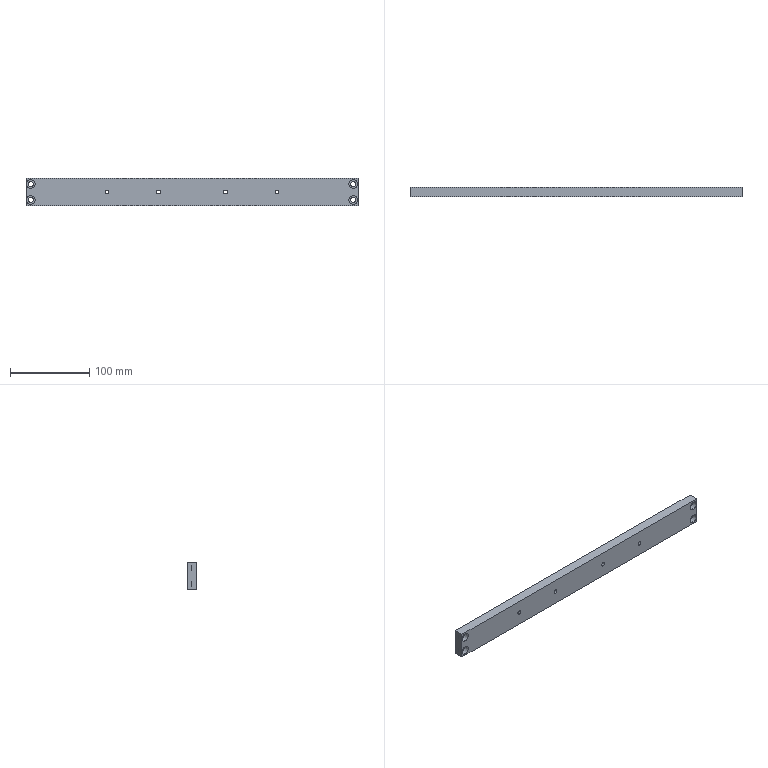Part | SolidWorks | features BaseBody 1 | 1 solid | 34 faces | box 420 x 12 x 35 mm | volume 172258 mm3 | cylinder 24 | plane 10 | commonest cylinder face diameters 5 x8 6.6 x8 11 x8
STEP:
#1=CARTESIAN_POINT('',(107.5,0.,-2.5));
#2=VERTEX_POINT('',#1);
#3=CARTESIAN_POINT('',(107.5,0.,2.5));
#4=VERTEX_POINT('',#3);
#5=CARTESIAN_POINT('',(107.5,0.,0.));
#6=DIRECTION('',(0.,1.,0.));
#7=DIRECTION('',(0.,0.,1.));
#8=AXIS2_PLACEMENT_3D('',#5,#6,#7);
#9=CIRCLE('',#8,2.5);
#10=EDGE_CURVE('',#2,#4,#9,.T.);
#11=ORIENTED_EDGE('',*,*,#10,.F.);
#12=CARTESIAN_POINT('',(107.5,12.,-2.5));
#13=VERTEX_POINT('',#12);
#14=CARTESIAN_POINT('',(107.5,12.,-2.5));
#15=DIRECTION('',(0.,1.,0.));
#16=VECTOR('',#15,1000.);
#17=LINE('',#14,#16);
#18=EDGE_CURVE('',#2,#13,#17,.T.);
#19=ORIENTED_EDGE('',*,*,#18,.T.);
#20=CARTESIAN_POINT('',(107.5,12.,2.5));
#21=VERTEX_POINT('',#20);
#22=CARTESIAN_POINT('',(107.5,12.,0.));
#23=DIRECTION('',(0.,1.,0.));
#24=DIRECTION('',(0.,0.,1.));
#25=AXIS2_PLACEMENT_3D('',#22,#23,#24);
#26=CIRCLE('',#25,2.5);
#27=EDGE_CURVE('',#13,#21,#26,.T.);
#28=ORIENTED_EDGE('',*,*,#27,.T.);
#29=CARTESIAN_POINT('',(107.5,12.,2.5));
#30=DIRECTION('',(0.,1.,0.));
#31=VECTOR('',#30,1000.);
#32=LINE('',#29,#31);
#33=EDGE_CURVE('',#4,#21,#32,.T.);
#34=ORIENTED_EDGE('',*,*,#33,.F.);
#35=EDGE_LOOP('',(#11,#19,#28,#34));
#36=FACE_OUTER_BOUND('',#35,.T.);
#37=CARTESIAN_POINT('',(107.5,12.,0.));
#38=DIRECTION('',(0.,1.,0.));
#39=DIRECTION('',(0.,0.,1.));
#40=AXIS2_PLACEMENT_3D('',#37,#38,#39);
#41=CYLINDRICAL_SURFACE('',#40,2.5);
#42=ADVANCED_FACE('',(#36),#41,.F.);
#43=CARTESIAN_POINT('',(42.5,0.,-2.5));
#44=VERTEX_POINT('',#43);
#45=CARTESIAN_POINT('',(42.5,0.,2.5));
#46=VERTEX_POINT('',#45);
#47=CARTESIAN_POINT('',(42.5,0.,0.));
#48=DIRECTION('',(0.,1.,0.));
#49=DIRECTION('',(0.,0.,1.));
#50=AXIS2_PLACEMENT_3D('',#47,#48,#49);
#51=CIRCLE('',#50,2.5);
#52=EDGE_CURVE('',#44,#46,#51,.T.);
#53=ORIENTED_EDGE('',*,*,#52,.F.);
#54=CARTESIAN_POINT('',(42.5,12.,-2.5));
#55=VERTEX_POINT('',#54);
#56=CARTESIAN_POINT('',(42.5,12.,-2.5));
#57=DIRECTION('',(0.,1.,0.));
#58=VECTOR('',#57,1000.);
#59=LINE('',#56,#58);
#60=EDGE_CURVE('',#44,#55,#59,.T.);
#61=ORIENTED_EDGE('',*,*,#60,.T.);
#62=CARTESIAN_POINT('',(42.5,12.,2.5));
#63=VERTEX_POINT('',#62);
#64=CARTESIAN_POINT('',(42.5,12.,0.));
#65=DIRECTION('',(0.,1.,0.));
#66=DIRECTION('',(0.,0.,1.));
#67=AXIS2_PLACEMENT_3D('',#64,#65,#66);
#68=CIRCLE('',#67,2.5);
#69=EDGE_CURVE('',#55,#63,#68,.T.);
#70=ORIENTED_EDGE('',*,*,#69,.T.);
#71=CARTESIAN_POINT('',(42.5,12.,2.5));
#72=DIRECTION('',(0.,1.,0.));
#73=VECTOR('',#72,1000.);
#74=LINE('',#71,#73);
#75=EDGE_CURVE('',#46,#63,#74,.T.);
#76=ORIENTED_EDGE('',*,*,#75,.F.);
#77=EDGE_LOOP('',(#53,#61,#70,#76));
#78=FACE_OUTER_BOUND('',#77,.T.);
#79=CARTESIAN_POINT('',(42.5,12.,0.));
#80=DIRECTION('',(0.,1.,0.));
#81=DIRECTION('',(0.,0.,1.));
#82=AXIS2_PLACEMENT_3D('',#79,#80,#81);
#83=CYLINDRICAL_SURFACE('',#82,2.5);
#84=ADVANCED_FACE('',(#78),#83,.F.);
#85=CARTESIAN_POINT('',(-42.5,0.,-2.5));
#86=VERTEX_POINT('',#85);
#87=CARTESIAN_POINT('',(-42.5,0.,2.5));
#88=VERTEX_POINT('',#87);
#89=CARTESIAN_POINT('',(-42.5,0.,0.));
#90=DIRECTION('',(0.,1.,0.));
#91=DIRECTION('',(0.,0.,1.));
#92=AXIS2_PLACEMENT_3D('',#89,#90,#91);
#93=CIRCLE('',#92,2.5);
#94=EDGE_CURVE('',#86,#88,#93,.T.);
#95=ORIENTED_EDGE('',*,*,#94,.F.);
#96=CARTESIAN_POINT('',(-42.5,12.,-2.5));
#97=VERTEX_POINT('',#96);
#98=CARTESIAN_POINT('',(-42.5,12.,-2.5));
#99=DIRECTION('',(0.,1.,0.));
#100=VECTOR('',#99,1000.);
#101=LINE('',#98,#100);
#102=EDGE_CURVE('',#86,#97,#101,.T.);
#103=ORIENTED_EDGE('',*,*,#102,.T.);
#104=CARTESIAN_POINT('',(-42.5,12.,2.5));
#105=VERTEX_POINT('',#104);
#106=CARTESIAN_POINT('',(-42.5,12.,0.));
#107=DIRECTION('',(0.,1.,0.));
#108=DIRECTION('',(0.,0.,1.));
#109=AXIS2_PLACEMENT_3D('',#106,#107,#108);
#110=CIRCLE('',#109,2.5);
#111=EDGE_CURVE('',#97,#105,#110,.T.);
#112=ORIENTED_EDGE('',*,*,#111,.T.);
#113=CARTESIAN_POINT('',(-42.5,12.,2.5));
#114=DIRECTION('',(0.,1.,0.));
#115=VECTOR('',#114,1000.);
#116=LINE('',#113,#115);
#117=EDGE_CURVE('',#88,#105,#116,.T.);
#118=ORIENTED_EDGE('',*,*,#117,.F.);
#119=EDGE_LOOP('',(#95,#103,#112,#118));
#120=FACE_OUTER_BOUND('',#119,.T.);
#121=CARTESIAN_POINT('',(-42.5,12.,0.));
#122=DIRECTION('',(0.,1.,0.));
#123=DIRECTION('',(0.,0.,1.));
#124=AXIS2_PLACEMENT_3D('',#121,#122,#123);
#125=CYLINDRICAL_SURFACE('',#124,2.5);
#126=ADVANCED_FACE('',(#120),#125,.F.);
#127=CARTESIAN_POINT('',(-107.5,0.,-2.5));
#128=VERTEX_POINT('',#127);
#129=CARTESIAN_POINT('',(-107.5,0.,2.5));
#130=VERTEX_POINT('',#129);
#131=CARTESIAN_POINT('',(-107.5,0.,0.));
#132=DIRECTION('',(0.,1.,0.));
#133=DIRECTION('',(0.,0.,1.));
#134=AXIS2_PLACEMENT_3D('',#131,#132,#133);
#135=CIRCLE('',#134,2.5);
#136=EDGE_CURVE('',#128,#130,#135,.T.);
#137=ORIENTED_EDGE('',*,*,#136,.F.);
#138=CARTESIAN_POINT('',(-107.5,12.,-2.5));
#139=VERTEX_POINT('',#138);
#140=CARTESIAN_POINT('',(-107.5,12.,-2.5));
#141=DIRECTION('',(0.,1.,0.));
#142=VECTOR('',#141,1000.);
#143=LINE('',#140,#142);
#144=EDGE_CURVE('',#128,#139,#143,.T.);
#145=ORIENTED_EDGE('',*,*,#144,.T.);
#146=CARTESIAN_POINT('',(-107.5,12.,2.5));
#147=VERTEX_POINT('',#146);
#148=CARTESIAN_POINT('',(-107.5,12.,0.));
#149=DIRECTION('',(0.,1.,0.));
#150=DIRECTION('',(0.,0.,1.));
#151=AXIS2_PLACEMENT_3D('',#148,#149,#150);
#152=CIRCLE('',#151,2.5);
#153=EDGE_CURVE('',#139,#147,#152,.T.);
#154=ORIENTED_EDGE('',*,*,#153,.T.);
#155=CARTESIAN_POINT('',(-107.5,12.,2.5));
#156=DIRECTION('',(0.,1.,0.));
#157=VECTOR('',#156,1000.);
#158=LINE('',#155,#157);
#159=EDGE_CURVE('',#130,#147,#158,.T.);
#160=ORIENTED_EDGE('',*,*,#159,.F.);
#161=EDGE_LOOP('',(#137,#145,#154,#160));
#162=FACE_OUTER_BOUND('',#161,.T.);
#163=CARTESIAN_POINT('',(-107.5,12.,0.));
#164=DIRECTION('',(0.,1.,0.));
#165=DIRECTION('',(0.,0.,1.));
#166=AXIS2_PLACEMENT_3D('',#163,#164,#165);
#167=CYLINDRICAL_SURFACE('',#166,2.5);
#168=ADVANCED_FACE('',(#162),#167,.F.);
#169=CARTESIAN_POINT('',(204.,6.4,-4.5));
#170=VERTEX_POINT('',#169);
#171=CARTESIAN_POINT('',(204.,6.4,-15.5));
#172=VERTEX_POINT('',#171);
#173=CARTESIAN_POINT('',(204.,6.4,-10.));
#174=DIRECTION('',(0.,-1.,0.));
#175=DIRECTION('',(0.,0.,-1.));
#176=AXIS2_PLACEMENT_3D('',#173,#174,#175);
#177=CIRCLE('',#176,5.5);
#178=EDGE_CURVE('',#170,#172,#177,.T.);
#179=ORIENTED_EDGE('',*,*,#178,.F.);
#180=CARTESIAN_POINT('',(204.,0.,-4.5));
#181=VERTEX_POINT('',#180);
#182=CARTESIAN_POINT('',(204.,0.,-4.5));
#183=DIRECTION('',(0.,-1.,0.));
#184=VECTOR('',#183,1000.);
#185=LINE('',#182,#184);
#186=EDGE_CURVE('',#170,#181,#185,.T.);
#187=ORIENTED_EDGE('',*,*,#186,.T.);
#188=CARTESIAN_POINT('',(204.,0.,-15.5));
#189=VERTEX_POINT('',#188);
#190=CARTESIAN_POINT('',(204.,0.,-10.));
#191=DIRECTION('',(0.,-1.,0.));
#192=DIRECTION('',(0.,0.,-1.));
#193=AXIS2_PLACEMENT_3D('',#190,#191,#192);
#194=CIRCLE('',#193,5.5);
#195=EDGE_CURVE('',#181,#189,#194,.T.);
#196=ORIENTED_EDGE('',*,*,#195,.T.);
#197=CARTESIAN_POINT('',(204.,0.,-15.5));
#198=DIRECTION('',(0.,-1.,0.));
#199=VECTOR('',#198,1000.);
#200=LINE('',#197,#199);
#201=EDGE_CURVE('',#172,#189,#200,.T.);
#202=ORIENTED_EDGE('',*,*,#201,.F.);
#203=EDGE_LOOP('',(#179,#187,#196,#202));
#204=FACE_OUTER_BOUND('',#203,.T.);
#205=CARTESIAN_POINT('',(204.,0.,-10.));
#206=DIRECTION('',(0.,-1.,0.));
#207=DIRECTION('',(0.,0.,-1.));
#208=AXIS2_PLACEMENT_3D('',#205,#206,#207);
#209=CYLINDRICAL_SURFACE('',#208,5.5);
#210=ADVANCED_FACE('',(#204),#209,.F.);
#211=CARTESIAN_POINT('',(204.,12.,-6.7));
#212=VERTEX_POINT('',#211);
#213=CARTESIAN_POINT('',(204.,12.,-13.3));
#214=VERTEX_POINT('',#213);
#215=CARTESIAN_POINT('',(204.,12.,-10.));
#216=DIRECTION('',(0.,-1.,0.));
#217=DIRECTION('',(0.,0.,-1.));
#218=AXIS2_PLACEMENT_3D('',#215,#216,#217);
#219=CIRCLE('',#218,3.3);
#220=EDGE_CURVE('',#212,#214,#219,.T.);
#221=ORIENTED_EDGE('',*,*,#220,.F.);
#222=CARTESIAN_POINT('',(204.,6.4,-6.7));
#223=VERTEX_POINT('',#222);
#224=CARTESIAN_POINT('',(204.,0.,-6.7));
#225=DIRECTION('',(0.,-1.,0.));
#226=VECTOR('',#225,1000.);
#227=LINE('',#224,#226);
#228=EDGE_CURVE('',#212,#223,#227,.T.);
#229=ORIENTED_EDGE('',*,*,#228,.T.);
#230=CARTESIAN_POINT('',(204.,6.4,-13.3));
#231=VERTEX_POINT('',#230);
#232=CARTESIAN_POINT('',(204.,6.4,-10.));
#233=DIRECTION('',(0.,-1.,0.));
#234=DIRECTION('',(0.,0.,-1.));
#235=AXIS2_PLACEMENT_3D('',#232,#233,#234);
#236=CIRCLE('',#235,3.3);
#237=EDGE_CURVE('',#223,#231,#236,.T.);
#238=ORIENTED_EDGE('',*,*,#237,.T.);
#239=CARTESIAN_POINT('',(204.,0.,-13.3));
#240=DIRECTION('',(0.,-1.,0.));
#241=VECTOR('',#240,1000.);
#242=LINE('',#239,#241);
#243=EDGE_CURVE('',#214,#231,#242,.T.);
#244=ORIENTED_EDGE('',*,*,#243,.F.);
#245=EDGE_LOOP('',(#221,#229,#238,#244));
#246=FACE_OUTER_BOUND('',#245,.T.);
#247=CARTESIAN_POINT('',(204.,0.,-10.));
#248=DIRECTION('',(0.,-1.,0.));
#249=DIRECTION('',(0.,0.,-1.));
#250=AXIS2_PLACEMENT_3D('',#247,#248,#249);
#251=CYLINDRICAL_SURFACE('',#250,3.3);
#252=ADVANCED_FACE('',(#246),#251,.F.);
#253=CARTESIAN_POINT('',(204.,6.4,15.5));
#254=VERTEX_POINT('',#253);
#255=CARTESIAN_POINT('',(204.,6.4,4.5));
#256=VERTEX_POINT('',#255);
#257=CARTESIAN_POINT('',(204.,6.4,10.));
#258=DIRECTION('',(0.,-1.,0.));
#259=DIRECTION('',(0.,0.,-1.));
#260=AXIS2_PLACEMENT_3D('',#257,#258,#259);
#261=CIRCLE('',#260,5.5);
#262=EDGE_CURVE('',#254,#256,#261,.T.);
#263=ORIENTED_EDGE('',*,*,#262,.F.);
#264=CARTESIAN_POINT('',(204.,0.,15.5));
#265=VERTEX_POINT('',#264);
#266=CARTESIAN_POINT('',(204.,0.,15.5));
#267=DIRECTION('',(0.,-1.,0.));
#268=VECTOR('',#267,1000.);
#269=LINE('',#266,#268);
#270=EDGE_CURVE('',#254,#265,#269,.T.);
#271=ORIENTED_EDGE('',*,*,#270,.T.);
#272=CARTESIAN_POINT('',(204.,0.,4.5));
#273=VERTEX_POINT('',#272);
#274=CARTESIAN_POINT('',(204.,0.,10.));
#275=DIRECTION('',(0.,-1.,0.));
#276=DIRECTION('',(0.,0.,-1.));
#277=AXIS2_PLACEMENT_3D('',#274,#275,#276);
#278=CIRCLE('',#277,5.5);
#279=EDGE_CURVE('',#265,#273,#278,.T.);
#280=ORIENTED_EDGE('',*,*,#279,.T.);
#281=CARTESIAN_POINT('',(204.,0.,4.5));
#282=DIRECTION('',(0.,-1.,0.));
#283=VECTOR('',#282,1000.);
#284=LINE('',#281,#283);
#285=EDGE_CURVE('',#256,#273,#284,.T.);
#286=ORIENTED_EDGE('',*,*,#285,.F.);
#287=EDGE_LOOP('',(#263,#271,#280,#286));
#288=FACE_OUTER_BOUND('',#287,.T.);
#289=CARTESIAN_POINT('',(204.,0.,10.));
#290=DIRECTION('',(0.,-1.,0.));
#291=DIRECTION('',(0.,0.,-1.));
#292=AXIS2_PLACEMENT_3D('',#289,#290,#291);
#293=CYLINDRICAL_SURFACE('',#292,5.5);
#294=ADVANCED_FACE('',(#288),#293,.F.);
#295=CARTESIAN_POINT('',(204.,12.,13.3));
#296=VERTEX_POINT('',#295);
#297=CARTESIAN_POINT('',(204.,12.,6.7));
#298=VERTEX_POINT('',#297);
#299=CARTESIAN_POINT('',(204.,12.,10.));
#300=DIRECTION('',(0.,-1.,0.));
#301=DIRECTION('',(0.,0.,-1.));
#302=AXIS2_PLACEMENT_3D('',#299,#300,#301);
#303=CIRCLE('',#302,3.3);
#304=EDGE_CURVE('',#296,#298,#303,.T.);
#305=ORIENTED_EDGE('',*,*,#304,.F.);
#306=CARTESIAN_POINT('',(204.,6.4,13.3));
#307=VERTEX_POINT('',#306);
#308=CARTESIAN_POINT('',(204.,0.,13.3));
#309=DIRECTION('',(0.,-1.,0.));
#310=VECTOR('',#309,1000.);
#311=LINE('',#308,#310);
#312=EDGE_CURVE('',#296,#307,#311,.T.);
#313=ORIENTED_EDGE('',*,*,#312,.T.);
#314=CARTESIAN_POINT('',(204.,6.4,6.7));
#315=VERTEX_POINT('',#314);
#316=CARTESIAN_POINT('',(204.,6.4,10.));
#317=DIRECTION('',(0.,-1.,0.));
#318=DIRECTION('',(0.,0.,-1.));
#319=AXIS2_PLACEMENT_3D('',#316,#317,#318);
#320=CIRCLE('',#319,3.3);
#321=EDGE_CURVE('',#307,#315,#320,.T.);
#322=ORIENTED_EDGE('',*,*,#321,.T.);
#323=CARTESIAN_POINT('',(204.,0.,6.7));
#324=DIRECTION('',(0.,-1.,0.));
#325=VECTOR('',#324,1000.);
#326=LINE('',#323,#325);
#327=EDGE_CURVE('',#298,#315,#326,.T.);
#328=ORIENTED_EDGE('',*,*,#327,.F.);
#329=EDGE_LOOP('',(#305,#313,#322,#328));
#330=FACE_OUTER_BOUND('',#329,.T.);
#331=CARTESIAN_POINT('',(204.,0.,10.));
#332=DIRECTION('',(0.,-1.,0.));
#333=DIRECTION('',(0.,0.,-1.));
#334=AXIS2_PLACEMENT_3D('',#331,#332,#333);
#335=CYLINDRICAL_SURFACE('',#334,3.3);
#336=ADVANCED_FACE('',(#330),#335,.F.);
#337=CARTESIAN_POINT('',(-204.,6.4,-4.5));
#338=VERTEX_POINT('',#337);
#339=CARTESIAN_POINT('',(-204.,6.4,-15.5));
#340=VERTEX_POINT('',#339);
#341=CARTESIAN_POINT('',(-204.,6.4,-10.));
#342=DIRECTION('',(0.,-1.,0.));
#343=DIRECTION('',(0.,0.,-1.));
#344=AXIS2_PLACEMENT_3D('',#341,#342,#343);
#345=CIRCLE('',#344,5.5);
#346=EDGE_CURVE('',#338,#340,#345,.T.);
#347=ORIENTED_EDGE('',*,*,#346,.F.);
#348=CARTESIAN_POINT('',(-204.,0.,-4.5));
#349=VERTEX_POINT('',#348);
#350=CARTESIAN_POINT('',(-204.,0.,-4.5));
#351=DIRECTION('',(0.,-1.,0.));
#352=VECTOR('',#351,1000.);
#353=LINE('',#350,#352);
#354=EDGE_CURVE('',#338,#349,#353,.T.);
#355=ORIENTED_EDGE('',*,*,#354,.T.);
#356=CARTESIAN_POINT('',(-204.,0.,-15.5));
#357=VERTEX_POINT('',#356);
#358=CARTESIAN_POINT('',(-204.,0.,-10.));
#359=DIRECTION('',(0.,-1.,0.));
#360=DIRECTION('',(0.,0.,-1.));
#361=AXIS2_PLACEMENT_3D('',#358,#359,#360);
#362=CIRCLE('',#361,5.5);
#363=EDGE_CURVE('',#349,#357,#362,.T.);
#364=ORIENTED_EDGE('',*,*,#363,.T.);
#365=CARTESIAN_POINT('',(-204.,0.,-15.5));
#366=DIRECTION('',(0.,-1.,0.));
#367=VECTOR('',#366,1000.);
#368=LINE('',#365,#367);
#369=EDGE_CURVE('',#340,#357,#368,.T.);
#370=ORIENTED_EDGE('',*,*,#369,.F.);
#371=EDGE_LOOP('',(#347,#355,#364,#370));
#372=FACE_OUTER_BOUND('',#371,.T.);
#373=CARTESIAN_POINT('',(-204.,0.,-10.));
#374=DIRECTION('',(0.,-1.,0.));
#375=DIRECTION('',(0.,0.,-1.));
#376=AXIS2_PLACEMENT_3D('',#373,#374,#375);
#377=CYLINDRICAL_SURFACE('',#376,5.5);
#378=ADVANCED_FACE('',(#372),#377,.F.);
#379=CARTESIAN_POINT('',(-204.,12.,-6.7));
#380=VERTEX_POINT('',#379);
#381=CARTESIAN_POINT('',(-204.,12.,-13.3));
#382=VERTEX_POINT('',#381);
#383=CARTESIAN_POINT('',(-204.,12.,-10.));
#384=DIRECTION('',(0.,-1.,0.));
#385=DIRECTION('',(0.,0.,-1.));
#386=AXIS2_PLACEMENT_3D('',#383,#384,#385);
#387=CIRCLE('',#386,3.3);
#388=EDGE_CURVE('',#380,#382,#387,.T.);
#389=ORIENTED_EDGE('',*,*,#388,.F.);
#390=CARTESIAN_POINT('',(-204.,6.4,-6.7));
#391=VERTEX_POINT('',#390);
#392=CARTESIAN_POINT('',(-204.,0.,-6.7));
#393=DIRECTION('',(0.,-1.,0.));
#394=VECTOR('',#393,1000.);
#395=LINE('',#392,#394);
#396=EDGE_CURVE('',#380,#391,#395,.T.);
#397=ORIENTED_EDGE('',*,*,#396,.T.);
#398=CARTESIAN_POINT('',(-204.,6.4,-13.3));
#399=VERTEX_POINT('',#398);
#400=CARTESIAN_POINT('',(-204.,6.4,-10.));
#401=DIRECTION('',(0.,-1.,0.));
#402=DIRECTION('',(0.,0.,-1.));
#403=AXIS2_PLACEMENT_3D('',#400,#401,#402);
#404=CIRCLE('',#403,3.3);
#405=EDGE_CURVE('',#391,#399,#404,.T.);
#406=ORIENTED_EDGE('',*,*,#405,.T.);
#407=CARTESIAN_POINT('',(-204.,0.,-13.3));
#408=DIRECTION('',(0.,-1.,0.));
#409=VECTOR('',#408,1000.);
#410=LINE('',#407,#409);
#411=EDGE_CURVE('',#382,#399,#410,.T.);
#412=ORIENTED_EDGE('',*,*,#411,.F.);
#413=EDGE_LOOP('',(#389,#397,#406,#412));
#414=FACE_OUTER_BOUND('',#413,.T.);
#415=CARTESIAN_POINT('',(-204.,0.,-10.));
#416=DIRECTION('',(0.,-1.,0.));
#417=DIRECTION('',(0.,0.,-1.));
#418=AXIS2_PLACEMENT_3D('',#415,#416,#417);
#419=CYLINDRICAL_SURFACE('',#418,3.3);
#420=ADVANCED_FACE('',(#414),#419,.F.);
#421=CARTESIAN_POINT('',(-204.,6.4,15.5));
#422=VERTEX_POINT('',#421);
#423=CARTESIAN_POINT('',(-204.,6.4,4.5));
#424=VERTEX_POINT('',#423);
#425=CARTESIAN_POINT('',(-204.,6.4,10.));
#426=DIRECTION('',(0.,-1.,0.));
#427=DIRECTION('',(0.,0.,-1.));
#428=AXIS2_PLACEMENT_3D('',#425,#426,#427);
#429=CIRCLE('',#428,5.5);
#430=EDGE_CURVE('',#422,#424,#429,.T.);
#431=ORIENTED_EDGE('',*,*,#430,.F.);
#432=CARTESIAN_POINT('',(-204.,0.,15.5));
#433=VERTEX_POINT('',#432);
#434=CARTESIAN_POINT('',(-204.,0.,15.5));
#435=DIRECTION('',(0.,-1.,0.));
#436=VECTOR('',#435,1000.);
#437=LINE('',#434,#436);
#438=EDGE_CURVE('',#422,#433,#437,.T.);
#439=ORIENTED_EDGE('',*,*,#438,.T.);
#440=CARTESIAN_POINT('',(-204.,0.,4.5));
#441=VERTEX_POINT('',#440);
#442=CARTESIAN_POINT('',(-204.,0.,10.));
#443=DIRECTION('',(0.,-1.,0.));
#444=DIRECTION('',(0.,0.,-1.));
#445=AXIS2_PLACEMENT_3D('',#442,#443,#444);
#446=CIRCLE('',#445,5.5);
#447=EDGE_CURVE('',#433,#441,#446,.T.);
#448=ORIENTED_EDGE('',*,*,#447,.T.);
#449=CARTESIAN_POINT('',(-204.,0.,4.5));
#450=DIRECTION('',(0.,-1.,0.));
#451=VECTOR('',#450,1000.);
#452=LINE('',#449,#451);
#453=EDGE_CURVE('',#424,#441,#452,.T.);
#454=ORIENTED_EDGE('',*,*,#453,.F.);
#455=EDGE_LOOP('',(#431,#439,#448,#454));
#456=FACE_OUTER_BOUND('',#455,.T.);
#457=CARTESIAN_POINT('',(-204.,0.,10.));
#458=DIRECTION('',(0.,-1.,0.));
#459=DIRECTION('',(0.,0.,-1.));
#460=AXIS2_PLACEMENT_3D('',#457,#458,#459);
#461=CYLINDRICAL_SURFACE('',#460,5.5);
#462=ADVANCED_FACE('',(#456),#461,.F.);
#463=CARTESIAN_POINT('',(-204.,12.,13.3));
#464=VERTEX_POINT('',#463);
#465=CARTESIAN_POINT('',(-204.,12.,6.7));
#466=VERTEX_POINT('',#465);
#467=CARTESIAN_POINT('',(-204.,12.,10.));
#468=DIRECTION('',(0.,-1.,0.));
#469=DIRECTION('',(0.,0.,-1.));
#470=AXIS2_PLACEMENT_3D('',#467,#468,#469);
#471=CIRCLE('',#470,3.3);
#472=EDGE_CURVE('',#464,#466,#471,.T.);
#473=ORIENTED_EDGE('',*,*,#472,.F.);
#474=CARTESIAN_POINT('',(-204.,6.4,13.3));
#475=VERTEX_POINT('',#474);
#476=CARTESIAN_POINT('',(-204.,0.,13.3));
#477=DIRECTION('',(0.,-1.,0.));
#478=VECTOR('',#477,1000.);
#479=LINE('',#476,#478);
#480=EDGE_CURVE('',#464,#475,#479,.T.);
#481=ORIENTED_EDGE('',*,*,#480,.T.);
#482=CARTESIAN_POINT('',(-204.,6.4,6.7));
#483=VERTEX_POINT('',#482);
#484=CARTESIAN_POINT('',(-204.,6.4,10.));
#485=DIRECTION('',(0.,-1.,0.));
#486=DIRECTION('',(0.,0.,-1.));
#487=AXIS2_PLACEMENT_3D('',#484,#485,#486);
#488=CIRCLE('',#487,3.3);
#489=EDGE_CURVE('',#475,#483,#488,.T.);
#490=ORIENTED_EDGE('',*,*,#489,.T.);
#491=CARTESIAN_POINT('',(-204.,0.,6.7));
#492=DIRECTION('',(0.,-1.,0.));
#493=VECTOR('',#492,1000.);
#494=LINE('',#491,#493);
#495=EDGE_CURVE('',#466,#483,#494,.T.);
#496=ORIENTED_EDGE('',*,*,#495,.F.);
#497=EDGE_LOOP('',(#473,#481,#490,#496));
#498=FACE_OUTER_BOUND('',#497,.T.);
#499=CARTESIAN_POINT('',(-204.,0.,10.));
#500=DIRECTION('',(0.,-1.,0.));
#501=DIRECTION('',(0.,0.,-1.));
#502=AXIS2_PLACEMENT_3D('',#499,#500,#501);
#503=CYLINDRICAL_SURFACE('',#502,3.3);
#504=ADVANCED_FACE('',(#498),#503,.F.);
#505=CARTESIAN_POINT('',(-210.,0.,-17.5));
#506=VERTEX_POINT('',#505);
#507=CARTESIAN_POINT('',(-210.,0.,17.5));
#508=VERTEX_POINT('',#507);
#509=CARTESIAN_POINT('',(-210.,0.,-17.5));
#510=DIRECTION('',(0.,0.,1.));
#511=VECTOR('',#510,1000.);
#512=LINE('',#509,#511);
#513=EDGE_CURVE('',#506,#508,#512,.T.);
#514=ORIENTED_EDGE('',*,*,#513,.T.);
#515=CARTESIAN_POINT('',(-210.,12.,17.5));
#516=VERTEX_POINT('',#515);
#517=CARTESIAN_POINT('',(-210.,12.,17.5));
#518=DIRECTION('',(0.,-1.,0.));
#519=VECTOR('',#518,1000.);
#520=LINE('',#517,#519);
#521=EDGE_CURVE('',#516,#508,#520,.T.);
#522=ORIENTED_EDGE('',*,*,#521,.F.);
#523=CARTESIAN_POINT('',(-210.,12.,-17.5));
#524=VERTEX_POINT('',#523);
#525=CARTESIAN_POINT('',(-210.,12.,-17.5));
#526=DIRECTION('',(0.,0.,1.));
#527=VECTOR('',#526,1000.);
#528=LINE('',#525,#527);
#529=EDGE_CURVE('',#524,#516,#528,.T.);
#530=ORIENTED_EDGE('',*,*,#529,.F.);
#531=CARTESIAN_POINT('',(-210.,12.,-17.5));
#532=DIRECTION('',(0.,-1.,0.));
#533=VECTOR('',#532,1000.);
#534=LINE('',#531,#533);
#535=EDGE_CURVE('',#524,#506,#534,.T.);
#536=ORIENTED_EDGE('',*,*,#535,.T.);
#537=EDGE_LOOP('',(#514,#522,#530,#536));
#538=FACE_OUTER_BOUND('',#537,.T.);
#539=CARTESIAN_POINT('',(-210.,12.,-17.5));
#540=DIRECTION('',(1.,0.,0.));
#541=DIRECTION('',(0.,0.,-1.));
#542=AXIS2_PLACEMENT_3D('',#539,#540,#541);
#543=PLANE('',#542);
#544=ADVANCED_FACE('',(#538),#543,.F.);
#545=CARTESIAN_POINT('',(210.,0.,17.5));
#546=VERTEX_POINT('',#545);
#547=CARTESIAN_POINT('',(210.,0.,17.5));
#548=DIRECTION('',(1.,0.,0.));
#549=VECTOR('',#548,1000.);
#550=LINE('',#547,#549);
#551=EDGE_CURVE('',#508,#546,#550,.T.);
#552=ORIENTED_EDGE('',*,*,#551,.T.);
#553=CARTESIAN_POINT('',(210.,12.,17.5));
#554=VERTEX_POINT('',#553);
#555=CARTESIAN_POINT('',(210.,12.,17.5));
#556=DIRECTION('',(0.,-1.,0.));
#557=VECTOR('',#556,1000.);
#558=LINE('',#555,#557);
#559=EDGE_CURVE('',#554,#546,#558,.T.);
#560=ORIENTED_EDGE('',*,*,#559,.F.);
#561=CARTESIAN_POINT('',(210.,12.,17.5));
#562=DIRECTION('',(1.,0.,0.));
#563=VECTOR('',#562,1000.);
#564=LINE('',#561,#563);
#565=EDGE_CURVE('',#516,#554,#564,.T.);
#566=ORIENTED_EDGE('',*,*,#565,.F.);
#567=ORIENTED_EDGE('',*,*,#521,.T.);
#568=EDGE_LOOP('',(#552,#560,#566,#567));
#569=FACE_OUTER_BOUND('',#568,.T.);
#570=CARTESIAN_POINT('',(210.,12.,17.5));
#571=DIRECTION('',(0.,0.,-1.));
#572=DIRECTION('',(-1.,0.,0.));
#573=AXIS2_PLACEMENT_3D('',#570,#571,#572);
#574=PLANE('',#573);
#575=ADVANCED_FACE('',(#569),#574,.F.);
#576=CARTESIAN_POINT('',(210.,0.,-17.5));
#577=VERTEX_POINT('',#576);
#578=CARTESIAN_POINT('',(210.,0.,-17.5));
#579=DIRECTION('',(0.,0.,-1.));
#580=VECTOR('',#579,1000.);
#581=LINE('',#578,#580);
#582=EDGE_CURVE('',#546,#577,#581,.T.);
#583=ORIENTED_EDGE('',*,*,#582,.T.);
#584=CARTESIAN_POINT('',(210.,12.,-17.5));
#585=VERTEX_POINT('',#584);
#586=CARTESIAN_POINT('',(210.,12.,-17.5));
#587=DIRECTION('',(0.,-1.,0.));
#588=VECTOR('',#587,1000.);
#589=LINE('',#586,#588);
#590=EDGE_CURVE('',#585,#577,#589,.T.);
#591=ORIENTED_EDGE('',*,*,#590,.F.);
#592=CARTESIAN_POINT('',(210.,12.,-17.5));
#593=DIRECTION('',(0.,0.,-1.));
#594=VECTOR('',#593,1000.);
#595=LINE('',#592,#594);
#596=EDGE_CURVE('',#554,#585,#595,.T.);
#597=ORIENTED_EDGE('',*,*,#596,.F.);
#598=ORIENTED_EDGE('',*,*,#559,.T.);
#599=EDGE_LOOP('',(#583,#591,#597,#598));
#600=FACE_OUTER_BOUND('',#599,.T.);
#601=CARTESIAN_POINT('',(210.,12.,-17.5));
#602=DIRECTION('',(-1.,0.,0.));
#603=DIRECTION('',(0.,0.,1.));
#604=AXIS2_PLACEMENT_3D('',#601,#602,#603);
#605=PLANE('',#604);
#606=ADVANCED_FACE('',(#600),#605,.F.);
#607=CARTESIAN_POINT('',(210.,0.,-17.5));
#608=DIRECTION('',(-1.,0.,0.));
#609=VECTOR('',#608,1000.);
#610=LINE('',#607,#609);
#611=EDGE_CURVE('',#577,#506,#610,.T.);
#612=ORIENTED_EDGE('',*,*,#611,.T.);
#613=ORIENTED_EDGE('',*,*,#535,.F.);
#614=CARTESIAN_POINT('',(210.,12.,-17.5));
#615=DIRECTION('',(-1.,0.,0.));
#616=VECTOR('',#615,1000.);
#617=LINE('',#614,#616);
#618=EDGE_CURVE('',#585,#524,#617,.T.);
#619=ORIENTED_EDGE('',*,*,#618,.F.);
#620=ORIENTED_EDGE('',*,*,#590,.T.);
#621=EDGE_LOOP('',(#612,#613,#619,#620));
#622=FACE_OUTER_BOUND('',#621,.T.);
#623=CARTESIAN_POINT('',(210.,12.,-17.5));
#624=DIRECTION('',(0.,0.,1.));
#625=DIRECTION('',(1.,0.,0.));
#626=AXIS2_PLACEMENT_3D('',#623,#624,#625);
#627=PLANE('',#626);
#628=ADVANCED_FACE('',(#622),#627,.F.);
#629=CARTESIAN_POINT('',(107.5,12.,0.));
#630=DIRECTION('',(0.,1.,0.));
#631=DIRECTION('',(0.,0.,1.));
#632=AXIS2_PLACEMENT_3D('',#629,#630,#631);
#633=CIRCLE('',#632,2.5);
#634=EDGE_CURVE('',#21,#13,#633,.T.);
#635=ORIENTED_EDGE('',*,*,#634,.F.);
#636=ORIENTED_EDGE('',*,*,#27,.F.);
#637=EDGE_LOOP('',(#635,#636));
#638=FACE_BOUND('',#637,.T.);
#639=CARTESIAN_POINT('',(42.5,12.,0.));
#640=DIRECTION('',(0.,1.,0.));
#641=DIRECTION('',(0.,0.,1.));
#642=AXIS2_PLACEMENT_3D('',#639,#640,#641);
#643=CIRCLE('',#642,2.5);
#644=EDGE_CURVE('',#63,#55,#643,.T.);
#645=ORIENTED_EDGE('',*,*,#644,.F.);
#646=ORIENTED_EDGE('',*,*,#69,.F.);
#647=EDGE_LOOP('',(#645,#646));
#648=FACE_BOUND('',#647,.T.);
#649=CARTESIAN_POINT('',(-42.5,12.,0.));
#650=DIRECTION('',(0.,1.,0.));
#651=DIRECTION('',(0.,0.,1.));
#652=AXIS2_PLACEMENT_3D('',#649,#650,#651);
#653=CIRCLE('',#652,2.5);
#654=EDGE_CURVE('',#105,#97,#653,.T.);
#655=ORIENTED_EDGE('',*,*,#654,.F.);
#656=ORIENTED_EDGE('',*,*,#111,.F.);
#657=EDGE_LOOP('',(#655,#656));
#658=FACE_BOUND('',#657,.T.);
#659=CARTESIAN_POINT('',(-107.5,12.,0.));
#660=DIRECTION('',(0.,1.,0.));
#661=DIRECTION('',(0.,0.,1.));
#662=AXIS2_PLACEMENT_3D('',#659,#660,#661);
#663=CIRCLE('',#662,2.5);
#664=EDGE_CURVE('',#147,#139,#663,.T.);
#665=ORIENTED_EDGE('',*,*,#664,.F.);
#666=ORIENTED_EDGE('',*,*,#153,.F.);
#667=EDGE_LOOP('',(#665,#666));
#668=FACE_BOUND('',#667,.T.);
#669=CARTESIAN_POINT('',(204.,12.,-10.));
#670=DIRECTION('',(0.,-1.,0.));
#671=DIRECTION('',(0.,0.,-1.));
#672=AXIS2_PLACEMENT_3D('',#669,#670,#671);
#673=CIRCLE('',#672,3.3);
#674=EDGE_CURVE('',#214,#212,#673,.T.);
#675=ORIENTED_EDGE('',*,*,#674,.T.);
#676=ORIENTED_EDGE('',*,*,#220,.T.);
#677=EDGE_LOOP('',(#675,#676));
#678=FACE_BOUND('',#677,.T.);
#679=CARTESIAN_POINT('',(204.,12.,10.));
#680=DIRECTION('',(0.,-1.,0.));
#681=DIRECTION('',(0.,0.,-1.));
#682=AXIS2_PLACEMENT_3D('',#679,#680,#681);
#683=CIRCLE('',#682,3.3);
#684=EDGE_CURVE('',#298,#296,#683,.T.);
#685=ORIENTED_EDGE('',*,*,#684,.T.);
#686=ORIENTED_EDGE('',*,*,#304,.T.);
#687=EDGE_LOOP('',(#685,#686));
#688=FACE_BOUND('',#687,.T.);
#689=CARTESIAN_POINT('',(-204.,12.,-10.));
#690=DIRECTION('',(0.,-1.,0.));
#691=DIRECTION('',(0.,0.,-1.));
#692=AXIS2_PLACEMENT_3D('',#689,#690,#691);
#693=CIRCLE('',#692,3.3);
#694=EDGE_CURVE('',#382,#380,#693,.T.);
#695=ORIENTED_EDGE('',*,*,#694,.T.);
#696=ORIENTED_EDGE('',*,*,#388,.T.);
#697=EDGE_LOOP('',(#695,#696));
#698=FACE_BOUND('',#697,.T.);
#699=CARTESIAN_POINT('',(-204.,12.,10.));
#700=DIRECTION('',(0.,-1.,0.));
#701=DIRECTION('',(0.,0.,-1.));
#702=AXIS2_PLACEMENT_3D('',#699,#700,#701);
#703=CIRCLE('',#702,3.3);
#704=EDGE_CURVE('',#466,#464,#703,.T.);
#705=ORIENTED_EDGE('',*,*,#704,.T.);
#706=ORIENTED_EDGE('',*,*,#472,.T.);
#707=EDGE_LOOP('',(#705,#706));
#708=FACE_BOUND('',#707,.T.);
#709=ORIENTED_EDGE('',*,*,#529,.T.);
#710=ORIENTED_EDGE('',*,*,#565,.T.);
#711=ORIENTED_EDGE('',*,*,#596,.T.);
#712=ORIENTED_EDGE('',*,*,#618,.T.);
#713=EDGE_LOOP('',(#709,#710,#711,#712));
#714=FACE_OUTER_BOUND('',#713,.T.);
#715=CARTESIAN_POINT('',(0.,12.,0.));
#716=DIRECTION('',(0.,-1.,0.));
#717=DIRECTION('',(0.,0.,-1.));
#718=AXIS2_PLACEMENT_3D('',#715,#716,#717);
#719=PLANE('',#718);
#720=ADVANCED_FACE('',(#638,#648,#658,#668,#678,#688,#698,#708,#714),#719,.F.);
#721=CARTESIAN_POINT('',(107.5,0.,0.));
#722=DIRECTION('',(0.,1.,0.));
#723=DIRECTION('',(0.,0.,1.));
#724=AXIS2_PLACEMENT_3D('',#721,#722,#723);
#725=CIRCLE('',#724,2.5);
#726=EDGE_CURVE('',#4,#2,#725,.T.);
#727=ORIENTED_EDGE('',*,*,#726,.T.);
#728=ORIENTED_EDGE('',*,*,#10,.T.);
#729=EDGE_LOOP('',(#727,#728));
#730=FACE_BOUND('',#729,.T.);
#731=CARTESIAN_POINT('',(42.5,0.,0.));
#732=DIRECTION('',(0.,1.,0.));
#733=DIRECTION('',(0.,0.,1.));
#734=AXIS2_PLACEMENT_3D('',#731,#732,#733);
#735=CIRCLE('',#734,2.5);
#736=EDGE_CURVE('',#46,#44,#735,.T.);
#737=ORIENTED_EDGE('',*,*,#736,.T.);
#738=ORIENTED_EDGE('',*,*,#52,.T.);
#739=EDGE_LOOP('',(#737,#738));
#740=FACE_BOUND('',#739,.T.);
#741=CARTESIAN_POINT('',(-42.5,0.,0.));
#742=DIRECTION('',(0.,1.,0.));
#743=DIRECTION('',(0.,0.,1.));
#744=AXIS2_PLACEMENT_3D('',#741,#742,#743);
#745=CIRCLE('',#744,2.5);
#746=EDGE_CURVE('',#88,#86,#745,.T.);
#747=ORIENTED_EDGE('',*,*,#746,.T.);
#748=ORIENTED_EDGE('',*,*,#94,.T.);
#749=EDGE_LOOP('',(#747,#748));
#750=FACE_BOUND('',#749,.T.);
#751=CARTESIAN_POINT('',(-107.5,0.,0.));
#752=DIRECTION('',(0.,1.,0.));
#753=DIRECTION('',(0.,0.,1.));
#754=AXIS2_PLACEMENT_3D('',#751,#752,#753);
#755=CIRCLE('',#754,2.5);
#756=EDGE_CURVE('',#130,#128,#755,.T.);
#757=ORIENTED_EDGE('',*,*,#756,.T.);
#758=ORIENTED_EDGE('',*,*,#136,.T.);
#759=EDGE_LOOP('',(#757,#758));
#760=FACE_BOUND('',#759,.T.);
#761=CARTESIAN_POINT('',(204.,0.,-10.));
#762=DIRECTION('',(0.,-1.,0.));
#763=DIRECTION('',(0.,0.,-1.));
#764=AXIS2_PLACEMENT_3D('',#761,#762,#763);
#765=CIRCLE('',#764,5.5);
#766=EDGE_CURVE('',#189,#181,#765,.T.);
#767=ORIENTED_EDGE('',*,*,#766,.F.);
#768=ORIENTED_EDGE('',*,*,#195,.F.);
#769=EDGE_LOOP('',(#767,#768));
#770=FACE_BOUND('',#769,.T.);
#771=CARTESIAN_POINT('',(204.,0.,10.));
#772=DIRECTION('',(0.,-1.,0.));
#773=DIRECTION('',(0.,0.,-1.));
#774=AXIS2_PLACEMENT_3D('',#771,#772,#773);
#775=CIRCLE('',#774,5.5);
#776=EDGE_CURVE('',#273,#265,#775,.T.);
#777=ORIENTED_EDGE('',*,*,#776,.F.);
#778=ORIENTED_EDGE('',*,*,#279,.F.);
#779=EDGE_LOOP('',(#777,#778));
#780=FACE_BOUND('',#779,.T.);
#781=CARTESIAN_POINT('',(-204.,0.,-10.));
#782=DIRECTION('',(0.,-1.,0.));
#783=DIRECTION('',(0.,0.,-1.));
#784=AXIS2_PLACEMENT_3D('',#781,#782,#783);
#785=CIRCLE('',#784,5.5);
#786=EDGE_CURVE('',#357,#349,#785,.T.);
#787=ORIENTED_EDGE('',*,*,#786,.F.);
#788=ORIENTED_EDGE('',*,*,#363,.F.);
#789=EDGE_LOOP('',(#787,#788));
#790=FACE_BOUND('',#789,.T.);
#791=CARTESIAN_POINT('',(-204.,0.,10.));
#792=DIRECTION('',(0.,-1.,0.));
#793=DIRECTION('',(0.,0.,-1.));
#794=AXIS2_PLACEMENT_3D('',#791,#792,#793);
#795=CIRCLE('',#794,5.5);
#796=EDGE_CURVE('',#441,#433,#795,.T.);
#797=ORIENTED_EDGE('',*,*,#796,.F.);
#798=ORIENTED_EDGE('',*,*,#447,.F.);
#799=EDGE_LOOP('',(#797,#798));
#800=FACE_BOUND('',#799,.T.);
#801=ORIENTED_EDGE('',*,*,#513,.F.);
#802=ORIENTED_EDGE('',*,*,#611,.F.);
#803=ORIENTED_EDGE('',*,*,#582,.F.);
#804=ORIENTED_EDGE('',*,*,#551,.F.);
#805=EDGE_LOOP('',(#801,#802,#803,#804));
#806=FACE_OUTER_BOUND('',#805,.T.);
#807=CARTESIAN_POINT('',(0.,0.,0.));
#808=DIRECTION('',(0.,-1.,0.));
#809=DIRECTION('',(0.,0.,-1.));
#810=AXIS2_PLACEMENT_3D('',#807,#808,#809);
#811=PLANE('',#810);
#812=ADVANCED_FACE('',(#730,#740,#750,#760,#770,#780,#790,#800,#806),#811,.T.);
#813=ORIENTED_EDGE('',*,*,#480,.F.);
#814=ORIENTED_EDGE('',*,*,#704,.F.);
#815=ORIENTED_EDGE('',*,*,#495,.T.);
#816=CARTESIAN_POINT('',(-204.,6.4,10.));
#817=DIRECTION('',(0.,-1.,0.));
#818=DIRECTION('',(0.,0.,-1.));
#819=AXIS2_PLACEMENT_3D('',#816,#817,#818);
#820=CIRCLE('',#819,3.3);
#821=EDGE_CURVE('',#483,#475,#820,.T.);
#822=ORIENTED_EDGE('',*,*,#821,.T.);
#823=EDGE_LOOP('',(#813,#814,#815,#822));
#824=FACE_OUTER_BOUND('',#823,.T.);
#825=CARTESIAN_POINT('',(-204.,0.,10.));
#826=DIRECTION('',(0.,-1.,0.));
#827=DIRECTION('',(0.,0.,-1.));
#828=AXIS2_PLACEMENT_3D('',#825,#826,#827);
#829=CYLINDRICAL_SURFACE('',#828,3.3);
#830=ADVANCED_FACE('',(#824),#829,.F.);
#831=ORIENTED_EDGE('',*,*,#821,.F.);
#832=ORIENTED_EDGE('',*,*,#489,.F.);
#833=EDGE_LOOP('',(#831,#832));
#834=FACE_BOUND('',#833,.T.);
#835=CARTESIAN_POINT('',(-204.,6.4,10.));
#836=DIRECTION('',(0.,-1.,0.));
#837=DIRECTION('',(0.,0.,-1.));
#838=AXIS2_PLACEMENT_3D('',#835,#836,#837);
#839=CIRCLE('',#838,5.5);
#840=EDGE_CURVE('',#424,#422,#839,.T.);
#841=ORIENTED_EDGE('',*,*,#840,.T.);
#842=ORIENTED_EDGE('',*,*,#430,.T.);
#843=EDGE_LOOP('',(#841,#842));
#844=FACE_OUTER_BOUND('',#843,.T.);
#845=CARTESIAN_POINT('',(-200.7,6.4,10.));
#846=DIRECTION('',(0.,1.,0.));
#847=DIRECTION('',(0.,0.,1.));
#848=AXIS2_PLACEMENT_3D('',#845,#846,#847);
#849=PLANE('',#848);
#850=ADVANCED_FACE('',(#834,#844),#849,.F.);
#851=ORIENTED_EDGE('',*,*,#438,.F.);
#852=ORIENTED_EDGE('',*,*,#840,.F.);
#853=ORIENTED_EDGE('',*,*,#453,.T.);
#854=ORIENTED_EDGE('',*,*,#796,.T.);
#855=EDGE_LOOP('',(#851,#852,#853,#854));
#856=FACE_OUTER_BOUND('',#855,.T.);
#857=CARTESIAN_POINT('',(-204.,0.,10.));
#858=DIRECTION('',(0.,-1.,0.));
#859=DIRECTION('',(0.,0.,-1.));
#860=AXIS2_PLACEMENT_3D('',#857,#858,#859);
#861=CYLINDRICAL_SURFACE('',#860,5.5);
#862=ADVANCED_FACE('',(#856),#861,.F.);
#863=ORIENTED_EDGE('',*,*,#396,.F.);
#864=ORIENTED_EDGE('',*,*,#694,.F.);
#865=ORIENTED_EDGE('',*,*,#411,.T.);
#866=CARTESIAN_POINT('',(-204.,6.4,-10.));
#867=DIRECTION('',(0.,-1.,0.));
#868=DIRECTION('',(0.,0.,-1.));
#869=AXIS2_PLACEMENT_3D('',#866,#867,#868);
#870=CIRCLE('',#869,3.3);
#871=EDGE_CURVE('',#399,#391,#870,.T.);
#872=ORIENTED_EDGE('',*,*,#871,.T.);
#873=EDGE_LOOP('',(#863,#864,#865,#872));
#874=FACE_OUTER_BOUND('',#873,.T.);
#875=CARTESIAN_POINT('',(-204.,0.,-10.));
#876=DIRECTION('',(0.,-1.,0.));
#877=DIRECTION('',(0.,0.,-1.));
#878=AXIS2_PLACEMENT_3D('',#875,#876,#877);
#879=CYLINDRICAL_SURFACE('',#878,3.3);
#880=ADVANCED_FACE('',(#874),#879,.F.);
#881=ORIENTED_EDGE('',*,*,#871,.F.);
#882=ORIENTED_EDGE('',*,*,#405,.F.);
#883=EDGE_LOOP('',(#881,#882));
#884=FACE_BOUND('',#883,.T.);
#885=CARTESIAN_POINT('',(-204.,6.4,-10.));
#886=DIRECTION('',(0.,-1.,0.));
#887=DIRECTION('',(0.,0.,-1.));
#888=AXIS2_PLACEMENT_3D('',#885,#886,#887);
#889=CIRCLE('',#888,5.5);
#890=EDGE_CURVE('',#340,#338,#889,.T.);
#891=ORIENTED_EDGE('',*,*,#890,.T.);
#892=ORIENTED_EDGE('',*,*,#346,.T.);
#893=EDGE_LOOP('',(#891,#892));
#894=FACE_OUTER_BOUND('',#893,.T.);
#895=CARTESIAN_POINT('',(-200.7,6.4,-10.));
#896=DIRECTION('',(0.,1.,0.));
#897=DIRECTION('',(0.,0.,1.));
#898=AXIS2_PLACEMENT_3D('',#895,#896,#897);
#899=PLANE('',#898);
#900=ADVANCED_FACE('',(#884,#894),#899,.F.);
#901=ORIENTED_EDGE('',*,*,#354,.F.);
#902=ORIENTED_EDGE('',*,*,#890,.F.);
#903=ORIENTED_EDGE('',*,*,#369,.T.);
#904=ORIENTED_EDGE('',*,*,#786,.T.);
#905=EDGE_LOOP('',(#901,#902,#903,#904));
#906=FACE_OUTER_BOUND('',#905,.T.);
#907=CARTESIAN_POINT('',(-204.,0.,-10.));
#908=DIRECTION('',(0.,-1.,0.));
#909=DIRECTION('',(0.,0.,-1.));
#910=AXIS2_PLACEMENT_3D('',#907,#908,#909);
#911=CYLINDRICAL_SURFACE('',#910,5.5);
#912=ADVANCED_FACE('',(#906),#911,.F.);
#913=ORIENTED_EDGE('',*,*,#312,.F.);
#914=ORIENTED_EDGE('',*,*,#684,.F.);
#915=ORIENTED_EDGE('',*,*,#327,.T.);
#916=CARTESIAN_POINT('',(204.,6.4,10.));
#917=DIRECTION('',(0.,-1.,0.));
#918=DIRECTION('',(0.,0.,-1.));
#919=AXIS2_PLACEMENT_3D('',#916,#917,#918);
#920=CIRCLE('',#919,3.3);
#921=EDGE_CURVE('',#315,#307,#920,.T.);
#922=ORIENTED_EDGE('',*,*,#921,.T.);
#923=EDGE_LOOP('',(#913,#914,#915,#922));
#924=FACE_OUTER_BOUND('',#923,.T.);
#925=CARTESIAN_POINT('',(204.,0.,10.));
#926=DIRECTION('',(0.,-1.,0.));
#927=DIRECTION('',(0.,0.,-1.));
#928=AXIS2_PLACEMENT_3D('',#925,#926,#927);
#929=CYLINDRICAL_SURFACE('',#928,3.3);
#930=ADVANCED_FACE('',(#924),#929,.F.);
#931=ORIENTED_EDGE('',*,*,#921,.F.);
#932=ORIENTED_EDGE('',*,*,#321,.F.);
#933=EDGE_LOOP('',(#931,#932));
#934=FACE_BOUND('',#933,.T.);
#935=CARTESIAN_POINT('',(204.,6.4,10.));
#936=DIRECTION('',(0.,-1.,0.));
#937=DIRECTION('',(0.,0.,-1.));
#938=AXIS2_PLACEMENT_3D('',#935,#936,#937);
#939=CIRCLE('',#938,5.5);
#940=EDGE_CURVE('',#256,#254,#939,.T.);
#941=ORIENTED_EDGE('',*,*,#940,.T.);
#942=ORIENTED_EDGE('',*,*,#262,.T.);
#943=EDGE_LOOP('',(#941,#942));
#944=FACE_OUTER_BOUND('',#943,.T.);
#945=CARTESIAN_POINT('',(207.3,6.4,10.));
#946=DIRECTION('',(0.,1.,0.));
#947=DIRECTION('',(0.,0.,1.));
#948=AXIS2_PLACEMENT_3D('',#945,#946,#947);
#949=PLANE('',#948);
#950=ADVANCED_FACE('',(#934,#944),#949,.F.);
#951=ORIENTED_EDGE('',*,*,#270,.F.);
#952=ORIENTED_EDGE('',*,*,#940,.F.);
#953=ORIENTED_EDGE('',*,*,#285,.T.);
#954=ORIENTED_EDGE('',*,*,#776,.T.);
#955=EDGE_LOOP('',(#951,#952,#953,#954));
#956=FACE_OUTER_BOUND('',#955,.T.);
#957=CARTESIAN_POINT('',(204.,0.,10.));
#958=DIRECTION('',(0.,-1.,0.));
#959=DIRECTION('',(0.,0.,-1.));
#960=AXIS2_PLACEMENT_3D('',#957,#958,#959);
#961=CYLINDRICAL_SURFACE('',#960,5.5);
#962=ADVANCED_FACE('',(#956),#961,.F.);
#963=ORIENTED_EDGE('',*,*,#228,.F.);
#964=ORIENTED_EDGE('',*,*,#674,.F.);
#965=ORIENTED_EDGE('',*,*,#243,.T.);
#966=CARTESIAN_POINT('',(204.,6.4,-10.));
#967=DIRECTION('',(0.,-1.,0.));
#968=DIRECTION('',(0.,0.,-1.));
#969=AXIS2_PLACEMENT_3D('',#966,#967,#968);
#970=CIRCLE('',#969,3.3);
#971=EDGE_CURVE('',#231,#223,#970,.T.);
#972=ORIENTED_EDGE('',*,*,#971,.T.);
#973=EDGE_LOOP('',(#963,#964,#965,#972));
#974=FACE_OUTER_BOUND('',#973,.T.);
#975=CARTESIAN_POINT('',(204.,0.,-10.));
#976=DIRECTION('',(0.,-1.,0.));
#977=DIRECTION('',(0.,0.,-1.));
#978=AXIS2_PLACEMENT_3D('',#975,#976,#977);
#979=CYLINDRICAL_SURFACE('',#978,3.3);
#980=ADVANCED_FACE('',(#974),#979,.F.);
#981=ORIENTED_EDGE('',*,*,#971,.F.);
#982=ORIENTED_EDGE('',*,*,#237,.F.);
#983=EDGE_LOOP('',(#981,#982));
#984=FACE_BOUND('',#983,.T.);
#985=CARTESIAN_POINT('',(204.,6.4,-10.));
#986=DIRECTION('',(0.,-1.,0.));
#987=DIRECTION('',(0.,0.,-1.));
#988=AXIS2_PLACEMENT_3D('',#985,#986,#987);
#989=CIRCLE('',#988,5.5);
#990=EDGE_CURVE('',#172,#170,#989,.T.);
#991=ORIENTED_EDGE('',*,*,#990,.T.);
#992=ORIENTED_EDGE('',*,*,#178,.T.);
#993=EDGE_LOOP('',(#991,#992));
#994=FACE_OUTER_BOUND('',#993,.T.);
#995=CARTESIAN_POINT('',(207.3,6.4,-10.));
#996=DIRECTION('',(0.,1.,0.));
#997=DIRECTION('',(0.,0.,1.));
#998=AXIS2_PLACEMENT_3D('',#995,#996,#997);
#999=PLANE('',#998);
#1000=ADVANCED_FACE('',(#984,#994),#999,.F.);
#1001=ORIENTED_EDGE('',*,*,#186,.F.);
#1002=ORIENTED_EDGE('',*,*,#990,.F.);
#1003=ORIENTED_EDGE('',*,*,#201,.T.);
#1004=ORIENTED_EDGE('',*,*,#766,.T.);
#1005=EDGE_LOOP('',(#1001,#1002,#1003,#1004));
#1006=FACE_OUTER_BOUND('',#1005,.T.);
#1007=CARTESIAN_POINT('',(204.,0.,-10.));
#1008=DIRECTION('',(0.,-1.,0.));
#1009=DIRECTION('',(0.,0.,-1.));
#1010=AXIS2_PLACEMENT_3D('',#1007,#1008,#1009);
#1011=CYLINDRICAL_SURFACE('',#1010,5.5);
#1012=ADVANCED_FACE('',(#1006),#1011,.F.);
#1013=ORIENTED_EDGE('',*,*,#144,.F.);
#1014=ORIENTED_EDGE('',*,*,#756,.F.);
#1015=ORIENTED_EDGE('',*,*,#159,.T.);
#1016=ORIENTED_EDGE('',*,*,#664,.T.);
#1017=EDGE_LOOP('',(#1013,#1014,#1015,#1016));
#1018=FACE_OUTER_BOUND('',#1017,.T.);
#1019=CARTESIAN_POINT('',(-107.5,12.,0.));
#1020=DIRECTION('',(0.,1.,0.));
#1021=DIRECTION('',(0.,0.,1.));
#1022=AXIS2_PLACEMENT_3D('',#1019,#1020,#1021);
#1023=CYLINDRICAL_SURFACE('',#1022,2.5);
#1024=ADVANCED_FACE('',(#1018),#1023,.F.);
#1025=ORIENTED_EDGE('',*,*,#102,.F.);
#1026=ORIENTED_EDGE('',*,*,#746,.F.);
#1027=ORIENTED_EDGE('',*,*,#117,.T.);
#1028=ORIENTED_EDGE('',*,*,#654,.T.);
#1029=EDGE_LOOP('',(#1025,#1026,#1027,#1028));
#1030=FACE_OUTER_BOUND('',#1029,.T.);
#1031=CARTESIAN_POINT('',(-42.5,12.,0.));
#1032=DIRECTION('',(0.,1.,0.));
#1033=DIRECTION('',(0.,0.,1.));
#1034=AXIS2_PLACEMENT_3D('',#1031,#1032,#1033);
#1035=CYLINDRICAL_SURFACE('',#1034,2.5);
#1036=ADVANCED_FACE('',(#1030),#1035,.F.);
#1037=ORIENTED_EDGE('',*,*,#60,.F.);
#1038=ORIENTED_EDGE('',*,*,#736,.F.);
#1039=ORIENTED_EDGE('',*,*,#75,.T.);
#1040=ORIENTED_EDGE('',*,*,#644,.T.);
#1041=EDGE_LOOP('',(#1037,#1038,#1039,#1040));
#1042=FACE_OUTER_BOUND('',#1041,.T.);
#1043=CARTESIAN_POINT('',(42.5,12.,0.));
#1044=DIRECTION('',(0.,1.,0.));
#1045=DIRECTION('',(0.,0.,1.));
#1046=AXIS2_PLACEMENT_3D('',#1043,#1044,#1045);
#1047=CYLINDRICAL_SURFACE('',#1046,2.5);
#1048=ADVANCED_FACE('',(#1042),#1047,.F.);
#1049=ORIENTED_EDGE('',*,*,#18,.F.);
#1050=ORIENTED_EDGE('',*,*,#726,.F.);
#1051=ORIENTED_EDGE('',*,*,#33,.T.);
#1052=ORIENTED_EDGE('',*,*,#634,.T.);
#1053=EDGE_LOOP('',(#1049,#1050,#1051,#1052));
#1054=FACE_OUTER_BOUND('',#1053,.T.);
#1055=CARTESIAN_POINT('',(107.5,12.,0.));
#1056=DIRECTION('',(0.,1.,0.));
#1057=DIRECTION('',(0.,0.,1.));
#1058=AXIS2_PLACEMENT_3D('',#1055,#1056,#1057);
#1059=CYLINDRICAL_SURFACE('',#1058,2.5);
#1060=ADVANCED_FACE('',(#1054),#1059,.F.);
#1061=CLOSED_SHELL('',(#42,#84,#126,#168,#210,#252,#294,#336,#378,#420,#462,#504,#544,#575,#606,#628,#720,#812,#830,#850,#862,#880,#900,#912,#930,#950,#962,#980,#1000,#1012,#1024,#1036,#1048,#1060));
#1062=MANIFOLD_SOLID_BREP('',#1061);
#1063=CARTESIAN_POINT('',(0.,0.,0.));
#1064=DIRECTION('',(0.,0.,1.));
#1065=DIRECTION('',(1.,0.,0.));
#1066=AXIS2_PLACEMENT_3D('',#1063,#1064,#1065);
#1067=(LENGTH_UNIT()NAMED_UNIT(*)SI_UNIT(.MILLI.,.METRE.));
#1068=UNCERTAINTY_MEASURE_WITH_UNIT(LENGTH_MEASURE(0.00001),#1067,'','');
#1069=(NAMED_UNIT(*)PLANE_ANGLE_UNIT()SI_UNIT($,.RADIAN.));
#1070=(NAMED_UNIT(*)SI_UNIT($,.STERADIAN.)SOLID_ANGLE_UNIT());
#1071=(GEOMETRIC_REPRESENTATION_CONTEXT(3)GLOBAL_UNCERTAINTY_ASSIGNED_CONTEXT((#1068))GLOBAL_UNIT_ASSIGNED_CONTEXT((#1067,#1069,#1070))REPRESENTATION_CONTEXT('',''));
#1072=ADVANCED_BREP_SHAPE_REPRESENTATION('',(#1062,#1066),#1071);